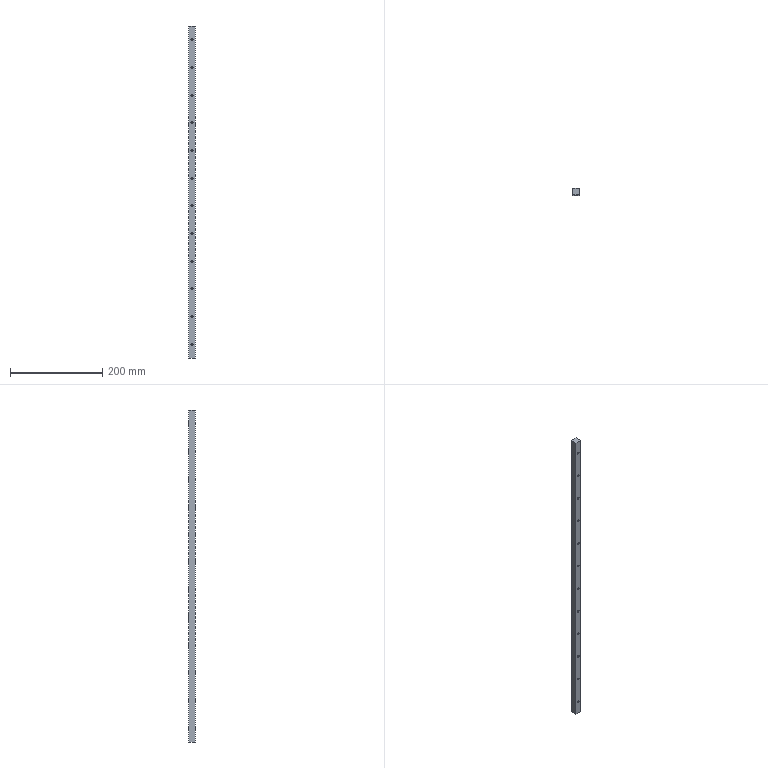Part | STEP file | PN_0064 (HGH15CA guide rail) | 1 solid | 66 faces | box 15 x 14 x 720 mm | volume 146714 mm3 | cylinder 48 | plane 18 | commonest cylinder face diameters 4.5 x24 8 x24